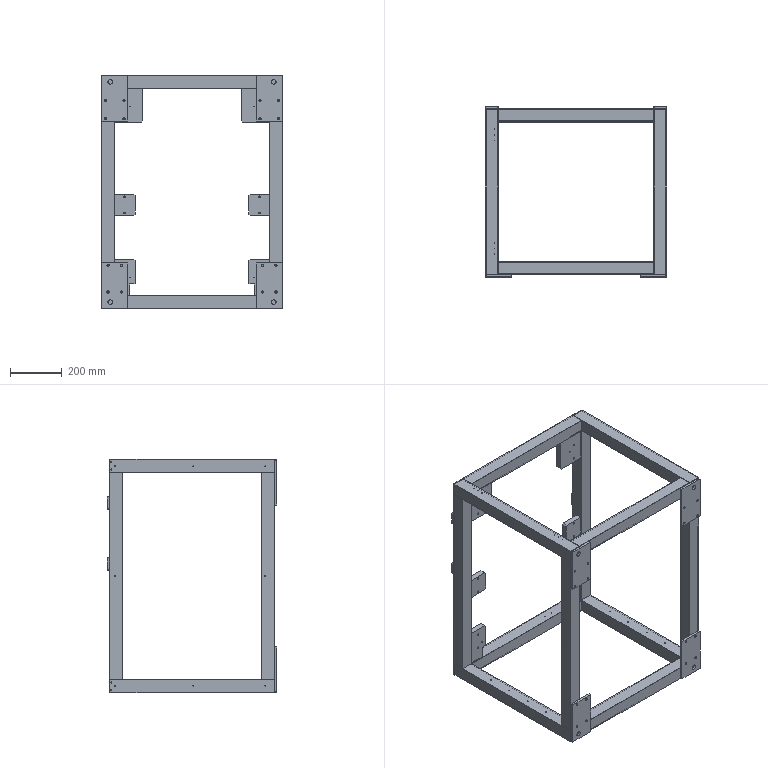Part | STEP file | 227H056111 Footstool Default | 26 solids | 572 faces | box 700 x 656 x 900 mm | volume 6881693 mm3 | plane 288 | cylinder 268 | cone 16 | commonest cylinder face diameters 4.2 x84 3.3 x60 8.5 x40 5 x32 6.8 x24 2.5 x20